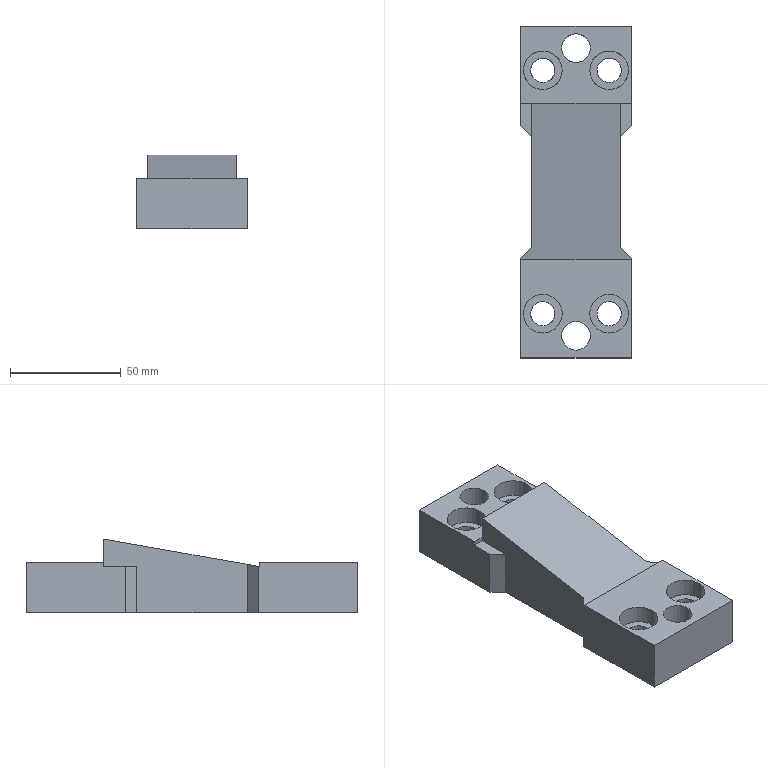Part | NX | features solid 2 | 1 solid | 36 faces | box 50 x 150 x 33.401 mm | volume 151864 mm3 | plane 26 | cylinder 10 | commonest cylinder face diameters 11 x4 17.5 x4 13 x2
STEP:
#1=CARTESIAN_POINT('',(-339.,-410.,-93.942));
#2=VERTEX_POINT('',#1);
#3=CARTESIAN_POINT('',(-339.,-410.329,-94.));
#4=VERTEX_POINT('',#3);
#5=CARTESIAN_POINT('',(-339.,-410.01,-93.944));
#6=DIRECTION('',(0.,-0.9848,-0.1736));
#7=VECTOR('',#6,1000.);
#8=LINE('',#5,#7);
#9=EDGE_CURVE('',#2,#4,#8,.T.);
#10=ORIENTED_EDGE('',*,*,#9,.F.);
#11=CARTESIAN_POINT('',(-339.,-410.,-115.));
#12=VERTEX_POINT('',#11);
#13=CARTESIAN_POINT('',(-339.,-410.,-94.));
#14=DIRECTION('',(0.,0.,-1.));
#15=VECTOR('',#14,1000.);
#16=LINE('',#13,#15);
#17=EDGE_CURVE('',#2,#12,#16,.T.);
#18=ORIENTED_EDGE('',*,*,#17,.T.);
#19=CARTESIAN_POINT('',(-339.,-455.,-115.));
#20=VERTEX_POINT('',#19);
#21=CARTESIAN_POINT('',(-339.,-410.,-115.));
#22=DIRECTION('',(0.,-1.,0.));
#23=VECTOR('',#22,1000.);
#24=LINE('',#21,#23);
#25=EDGE_CURVE('',#12,#20,#24,.T.);
#26=ORIENTED_EDGE('',*,*,#25,.T.);
#27=CARTESIAN_POINT('',(-339.,-455.,-92.));
#28=VERTEX_POINT('',#27);
#29=CARTESIAN_POINT('',(-339.,-455.,-94.));
#30=DIRECTION('',(0.,0.,-1.));
#31=VECTOR('',#30,1000.);
#32=LINE('',#29,#31);
#33=EDGE_CURVE('',#28,#20,#32,.T.);
#34=ORIENTED_EDGE('',*,*,#33,.F.);
#35=CARTESIAN_POINT('',(-339.,-410.329,-92.));
#36=VERTEX_POINT('',#35);
#37=CARTESIAN_POINT('',(-339.,-410.,-92.));
#38=DIRECTION('',(0.,-1.,0.));
#39=VECTOR('',#38,1000.);
#40=LINE('',#37,#39);
#41=EDGE_CURVE('',#36,#28,#40,.T.);
#42=ORIENTED_EDGE('',*,*,#41,.F.);
#43=CARTESIAN_POINT('',(-339.,-410.329,-94.));
#44=DIRECTION('',(0.,0.,-1.));
#45=VECTOR('',#44,1000.);
#46=LINE('',#43,#45);
#47=EDGE_CURVE('',#36,#4,#46,.T.);
#48=ORIENTED_EDGE('',*,*,#47,.T.);
#49=EDGE_LOOP('',(#10,#18,#26,#34,#42,#48));
#50=FACE_BOUND('',#49,.T.);
#51=CARTESIAN_POINT('',(-339.,-410.,-94.));
#52=DIRECTION('',(1.,0.,0.));
#53=DIRECTION('',(0.,1.,0.));
#54=AXIS2_PLACEMENT_3D('',#51,#52,#53);
#55=PLANE('',#54);
#56=ADVANCED_FACE('',(#50),#55,.F.);
#57=CARTESIAN_POINT('',(-334.,-405.,-93.06));
#58=VERTEX_POINT('',#57);
#59=CARTESIAN_POINT('',(-334.082,-405.082,-93.075));
#60=DIRECTION('',(-0.7017,-0.7017,-0.1237));
#61=VECTOR('',#60,1000.);
#62=LINE('',#59,#61);
#63=EDGE_CURVE('',#58,#2,#62,.T.);
#64=ORIENTED_EDGE('',*,*,#63,.F.);
#65=CARTESIAN_POINT('',(-334.,-405.,-115.));
#66=VERTEX_POINT('',#65);
#67=CARTESIAN_POINT('',(-334.,-405.,-94.));
#68=DIRECTION('',(0.,0.,-1.));
#69=VECTOR('',#68,1000.);
#70=LINE('',#67,#69);
#71=EDGE_CURVE('',#58,#66,#70,.T.);
#72=ORIENTED_EDGE('',*,*,#71,.T.);
#73=CARTESIAN_POINT('',(-334.,-405.,-115.));
#74=DIRECTION('',(-0.7071,-0.7071,0.));
#75=VECTOR('',#74,1000.);
#76=LINE('',#73,#75);
#77=EDGE_CURVE('',#66,#12,#76,.T.);
#78=ORIENTED_EDGE('',*,*,#77,.T.);
#79=ORIENTED_EDGE('',*,*,#17,.F.);
#80=EDGE_LOOP('',(#64,#72,#78,#79));
#81=FACE_BOUND('',#80,.T.);
#82=CARTESIAN_POINT('',(-334.,-405.,-94.));
#83=DIRECTION('',(0.7071,-0.7071,0.));
#84=DIRECTION('',(0.7071,0.7071,0.));
#85=AXIS2_PLACEMENT_3D('',#82,#83,#84);
#86=PLANE('',#85);
#87=ADVANCED_FACE('',(#81),#86,.F.);
#88=CARTESIAN_POINT('',(-329.,-443.75,-92.));
#89=VERTEX_POINT('',#88);
#90=CARTESIAN_POINT('',(-329.,-435.,-92.));
#91=DIRECTION('',(0.,0.,1.));
#92=DIRECTION('',(0.,-1.,0.));
#93=AXIS2_PLACEMENT_3D('',#90,#91,#92);
#94=CIRCLE('',#93,8.75);
#95=EDGE_CURVE('',#89,#89,#94,.T.);
#96=ORIENTED_EDGE('',*,*,#95,.F.);
#97=EDGE_LOOP('',(#96));
#98=FACE_BOUND('',#97,.T.);
#99=CARTESIAN_POINT('',(-314.,-451.5,-92.));
#100=VERTEX_POINT('',#99);
#101=CARTESIAN_POINT('',(-314.,-445.,-92.));
#102=DIRECTION('',(0.,0.,1.));
#103=DIRECTION('',(0.,-1.,0.));
#104=AXIS2_PLACEMENT_3D('',#101,#102,#103);
#105=CIRCLE('',#104,6.5);
#106=EDGE_CURVE('',#100,#100,#105,.T.);
#107=ORIENTED_EDGE('',*,*,#106,.F.);
#108=EDGE_LOOP('',(#107));
#109=FACE_BOUND('',#108,.T.);
#110=CARTESIAN_POINT('',(-299.,-443.75,-92.));
#111=VERTEX_POINT('',#110);
#112=CARTESIAN_POINT('',(-299.,-435.,-92.));
#113=DIRECTION('',(0.,0.,1.));
#114=DIRECTION('',(0.,-1.,0.));
#115=AXIS2_PLACEMENT_3D('',#112,#113,#114);
#116=CIRCLE('',#115,8.75);
#117=EDGE_CURVE('',#111,#111,#116,.T.);
#118=ORIENTED_EDGE('',*,*,#117,.F.);
#119=EDGE_LOOP('',(#118));
#120=FACE_BOUND('',#119,.T.);
#121=CARTESIAN_POINT('',(-289.,-410.329,-92.));
#122=VERTEX_POINT('',#121);
#123=CARTESIAN_POINT('',(-294.,-410.329,-92.));
#124=DIRECTION('',(-1.,0.,0.));
#125=VECTOR('',#124,1000.);
#126=LINE('',#123,#125);
#127=EDGE_CURVE('',#122,#36,#126,.T.);
#128=ORIENTED_EDGE('',*,*,#127,.T.);
#129=ORIENTED_EDGE('',*,*,#41,.T.);
#130=CARTESIAN_POINT('',(-289.,-455.,-92.));
#131=VERTEX_POINT('',#130);
#132=CARTESIAN_POINT('',(-289.,-455.,-92.));
#133=DIRECTION('',(-1.,0.,0.));
#134=VECTOR('',#133,1000.);
#135=LINE('',#132,#134);
#136=EDGE_CURVE('',#131,#28,#135,.T.);
#137=ORIENTED_EDGE('',*,*,#136,.F.);
#138=CARTESIAN_POINT('',(-289.,-410.,-92.));
#139=DIRECTION('',(0.,-1.,0.));
#140=VECTOR('',#139,1000.);
#141=LINE('',#138,#140);
#142=EDGE_CURVE('',#122,#131,#141,.T.);
#143=ORIENTED_EDGE('',*,*,#142,.F.);
#144=EDGE_LOOP('',(#128,#129,#137,#143));
#145=FACE_BOUND('',#144,.T.);
#146=CARTESIAN_POINT('',(-289.,-305.,-92.));
#147=DIRECTION('',(0.,0.,-1.));
#148=DIRECTION('',(1.,0.,0.));
#149=AXIS2_PLACEMENT_3D('',#146,#147,#148);
#150=PLANE('',#149);
#151=ADVANCED_FACE('',(#98,#109,#120,#145),#150,.F.);
#152=ORIENTED_EDGE('',*,*,#71,.F.);
#153=CARTESIAN_POINT('',(-334.,-340.,-81.599));
#154=VERTEX_POINT('',#153);
#155=CARTESIAN_POINT('',(-334.,-340.,-81.599));
#156=DIRECTION('',(0.,-0.9848,-0.1736));
#157=VECTOR('',#156,1000.);
#158=LINE('',#155,#157);
#159=EDGE_CURVE('',#154,#58,#158,.T.);
#160=ORIENTED_EDGE('',*,*,#159,.F.);
#161=CARTESIAN_POINT('',(-334.,-340.,-92.));
#162=VERTEX_POINT('',#161);
#163=CARTESIAN_POINT('',(-334.,-340.,-81.599));
#164=DIRECTION('',(0.,0.,-1.));
#165=VECTOR('',#164,1000.);
#166=LINE('',#163,#165);
#167=EDGE_CURVE('',#154,#162,#166,.T.);
#168=ORIENTED_EDGE('',*,*,#167,.T.);
#169=CARTESIAN_POINT('',(-334.,-340.,-94.));
#170=VERTEX_POINT('',#169);
#171=CARTESIAN_POINT('',(-334.,-340.,-81.599));
#172=DIRECTION('',(0.,0.,-1.));
#173=VECTOR('',#172,1000.);
#174=LINE('',#171,#173);
#175=EDGE_CURVE('',#162,#170,#174,.T.);
#176=ORIENTED_EDGE('',*,*,#175,.T.);
#177=CARTESIAN_POINT('',(-334.,-355.,-94.));
#178=VERTEX_POINT('',#177);
#179=CARTESIAN_POINT('',(-334.,-340.,-94.));
#180=DIRECTION('',(0.,-1.,0.));
#181=VECTOR('',#180,1000.);
#182=LINE('',#179,#181);
#183=EDGE_CURVE('',#170,#178,#182,.T.);
#184=ORIENTED_EDGE('',*,*,#183,.T.);
#185=CARTESIAN_POINT('',(-334.,-355.,-115.));
#186=VERTEX_POINT('',#185);
#187=CARTESIAN_POINT('',(-334.,-355.,-94.));
#188=DIRECTION('',(0.,0.,-1.));
#189=VECTOR('',#188,1000.);
#190=LINE('',#187,#189);
#191=EDGE_CURVE('',#178,#186,#190,.T.);
#192=ORIENTED_EDGE('',*,*,#191,.T.);
#193=CARTESIAN_POINT('',(-334.,-355.,-115.));
#194=DIRECTION('',(0.,-1.,0.));
#195=VECTOR('',#194,1000.);
#196=LINE('',#193,#195);
#197=EDGE_CURVE('',#186,#66,#196,.T.);
#198=ORIENTED_EDGE('',*,*,#197,.T.);
#199=EDGE_LOOP('',(#152,#160,#168,#176,#184,#192,#198));
#200=FACE_BOUND('',#199,.T.);
#201=CARTESIAN_POINT('',(-334.,-355.,-94.));
#202=DIRECTION('',(1.,0.,0.));
#203=DIRECTION('',(0.,1.,0.));
#204=AXIS2_PLACEMENT_3D('',#201,#202,#203);
#205=PLANE('',#204);
#206=ADVANCED_FACE('',(#200),#205,.F.);
#207=CARTESIAN_POINT('',(-294.,-340.,-81.599));
#208=VERTEX_POINT('',#207);
#209=CARTESIAN_POINT('',(-294.,-340.,-92.));
#210=VERTEX_POINT('',#209);
#211=CARTESIAN_POINT('',(-294.,-340.,-81.599));
#212=DIRECTION('',(0.,0.,-1.));
#213=VECTOR('',#212,1000.);
#214=LINE('',#211,#213);
#215=EDGE_CURVE('',#208,#210,#214,.T.);
#216=ORIENTED_EDGE('',*,*,#215,.T.);
#217=CARTESIAN_POINT('',(-294.,-340.,-92.));
#218=DIRECTION('',(-1.,0.,0.));
#219=VECTOR('',#218,1000.);
#220=LINE('',#217,#219);
#221=EDGE_CURVE('',#210,#162,#220,.T.);
#222=ORIENTED_EDGE('',*,*,#221,.T.);
#223=ORIENTED_EDGE('',*,*,#167,.F.);
#224=CARTESIAN_POINT('',(-294.,-340.,-81.599));
#225=DIRECTION('',(-1.,0.,0.));
#226=VECTOR('',#225,1000.);
#227=LINE('',#224,#226);
#228=EDGE_CURVE('',#208,#154,#227,.T.);
#229=ORIENTED_EDGE('',*,*,#228,.F.);
#230=EDGE_LOOP('',(#216,#222,#223,#229));
#231=FACE_BOUND('',#230,.T.);
#232=CARTESIAN_POINT('',(-294.,-340.,-81.599));
#233=DIRECTION('',(0.,1.,0.));
#234=DIRECTION('',(-1.,0.,0.));
#235=AXIS2_PLACEMENT_3D('',#232,#233,#234);
#236=PLANE('',#235);
#237=ADVANCED_FACE('',(#231),#236,.T.);
#238=ORIENTED_EDGE('',*,*,#183,.F.);
#239=CARTESIAN_POINT('',(-339.,-340.,-94.));
#240=VERTEX_POINT('',#239);
#241=CARTESIAN_POINT('',(-289.,-340.,-94.));
#242=DIRECTION('',(-1.,0.,0.));
#243=VECTOR('',#242,1000.);
#244=LINE('',#241,#243);
#245=EDGE_CURVE('',#170,#240,#244,.T.);
#246=ORIENTED_EDGE('',*,*,#245,.T.);
#247=CARTESIAN_POINT('',(-339.,-350.,-94.));
#248=VERTEX_POINT('',#247);
#249=CARTESIAN_POINT('',(-339.,-305.,-94.));
#250=DIRECTION('',(0.,-1.,0.));
#251=VECTOR('',#250,1000.);
#252=LINE('',#249,#251);
#253=EDGE_CURVE('',#240,#248,#252,.T.);
#254=ORIENTED_EDGE('',*,*,#253,.T.);
#255=CARTESIAN_POINT('',(-334.,-355.,-94.));
#256=DIRECTION('',(-0.7071,0.7071,0.));
#257=VECTOR('',#256,1000.);
#258=LINE('',#255,#257);
#259=EDGE_CURVE('',#178,#248,#258,.T.);
#260=ORIENTED_EDGE('',*,*,#259,.F.);
#261=EDGE_LOOP('',(#238,#246,#254,#260));
#262=FACE_BOUND('',#261,.T.);
#263=CARTESIAN_POINT('',(-289.,-305.,-94.));
#264=DIRECTION('',(0.,0.,-1.));
#265=DIRECTION('',(1.,0.,0.));
#266=AXIS2_PLACEMENT_3D('',#263,#264,#265);
#267=PLANE('',#266);
#268=ADVANCED_FACE('',(#262),#267,.F.);
#269=CARTESIAN_POINT('',(-289.,-340.,-94.));
#270=VERTEX_POINT('',#269);
#271=CARTESIAN_POINT('',(-294.,-340.,-94.));
#272=VERTEX_POINT('',#271);
#273=CARTESIAN_POINT('',(-289.,-340.,-94.));
#274=DIRECTION('',(-1.,0.,0.));
#275=VECTOR('',#274,1000.);
#276=LINE('',#273,#275);
#277=EDGE_CURVE('',#270,#272,#276,.T.);
#278=ORIENTED_EDGE('',*,*,#277,.T.);
#279=CARTESIAN_POINT('',(-294.,-355.,-94.));
#280=VERTEX_POINT('',#279);
#281=CARTESIAN_POINT('',(-294.,-340.,-94.));
#282=DIRECTION('',(0.,-1.,0.));
#283=VECTOR('',#282,1000.);
#284=LINE('',#281,#283);
#285=EDGE_CURVE('',#272,#280,#284,.T.);
#286=ORIENTED_EDGE('',*,*,#285,.T.);
#287=CARTESIAN_POINT('',(-289.,-350.,-94.));
#288=VERTEX_POINT('',#287);
#289=CARTESIAN_POINT('',(-289.,-350.,-94.));
#290=DIRECTION('',(-0.7071,-0.7071,0.));
#291=VECTOR('',#290,1000.);
#292=LINE('',#289,#291);
#293=EDGE_CURVE('',#288,#280,#292,.T.);
#294=ORIENTED_EDGE('',*,*,#293,.F.);
#295=CARTESIAN_POINT('',(-289.,-305.,-94.));
#296=DIRECTION('',(0.,-1.,0.));
#297=VECTOR('',#296,1000.);
#298=LINE('',#295,#297);
#299=EDGE_CURVE('',#270,#288,#298,.T.);
#300=ORIENTED_EDGE('',*,*,#299,.F.);
#301=EDGE_LOOP('',(#278,#286,#294,#300));
#302=FACE_BOUND('',#301,.T.);
#303=CARTESIAN_POINT('',(-289.,-305.,-94.));
#304=DIRECTION('',(0.,0.,-1.));
#305=DIRECTION('',(1.,0.,0.));
#306=AXIS2_PLACEMENT_3D('',#303,#304,#305);
#307=PLANE('',#306);
#308=ADVANCED_FACE('',(#302),#307,.F.);
#309=ORIENTED_EDGE('',*,*,#245,.F.);
#310=ORIENTED_EDGE('',*,*,#175,.F.);
#311=CARTESIAN_POINT('',(-339.,-340.,-92.));
#312=VERTEX_POINT('',#311);
#313=CARTESIAN_POINT('',(-289.,-340.,-92.));
#314=DIRECTION('',(-1.,0.,0.));
#315=VECTOR('',#314,1000.);
#316=LINE('',#313,#315);
#317=EDGE_CURVE('',#162,#312,#316,.T.);
#318=ORIENTED_EDGE('',*,*,#317,.T.);
#319=CARTESIAN_POINT('',(-339.,-340.,-94.));
#320=DIRECTION('',(0.,0.,-1.));
#321=VECTOR('',#320,1000.);
#322=LINE('',#319,#321);
#323=EDGE_CURVE('',#312,#240,#322,.T.);
#324=ORIENTED_EDGE('',*,*,#323,.T.);
#325=EDGE_LOOP('',(#309,#310,#318,#324));
#326=FACE_BOUND('',#325,.T.);
#327=CARTESIAN_POINT('',(-289.,-340.,-75.44));
#328=DIRECTION('',(0.,-1.,0.));
#329=DIRECTION('',(1.,0.,0.));
#330=AXIS2_PLACEMENT_3D('',#327,#328,#329);
#331=PLANE('',#330);
#332=ADVANCED_FACE('',(#326),#331,.T.);
#333=CARTESIAN_POINT('',(-329.,-440.5,-115.));
#334=VERTEX_POINT('',#333);
#335=CARTESIAN_POINT('',(-329.,-435.,-115.));
#336=DIRECTION('',(0.,0.,1.));
#337=DIRECTION('',(0.,-1.,0.));
#338=AXIS2_PLACEMENT_3D('',#335,#336,#337);
#339=CIRCLE('',#338,5.5);
#340=EDGE_CURVE('',#334,#334,#339,.T.);
#341=ORIENTED_EDGE('',*,*,#340,.F.);
#342=EDGE_LOOP('',(#341));
#343=FACE_BOUND('',#342,.T.);
#344=CARTESIAN_POINT('',(-334.5,-435.,-100.));
#345=VERTEX_POINT('',#344);
#346=CARTESIAN_POINT('',(-329.,-435.,-100.));
#347=DIRECTION('',(0.,0.,1.));
#348=DIRECTION('',(-1.,0.,0.));
#349=AXIS2_PLACEMENT_3D('',#346,#347,#348);
#350=CIRCLE('',#349,5.5);
#351=EDGE_CURVE('',#345,#345,#350,.T.);
#352=ORIENTED_EDGE('',*,*,#351,.T.);
#353=EDGE_LOOP('',(#352));
#354=FACE_BOUND('',#353,.T.);
#355=CARTESIAN_POINT('',(-329.,-435.,-94.));
#356=DIRECTION('',(0.,0.,-1.));
#357=DIRECTION('',(1.,0.,0.));
#358=AXIS2_PLACEMENT_3D('',#355,#356,#357);
#359=CYLINDRICAL_SURFACE('',#358,5.5);
#360=ADVANCED_FACE('',(#343,#354),#359,.F.);
#361=CARTESIAN_POINT('',(-299.,-440.5,-115.));
#362=VERTEX_POINT('',#361);
#363=CARTESIAN_POINT('',(-299.,-435.,-115.));
#364=DIRECTION('',(0.,0.,1.));
#365=DIRECTION('',(0.,-1.,0.));
#366=AXIS2_PLACEMENT_3D('',#363,#364,#365);
#367=CIRCLE('',#366,5.5);
#368=EDGE_CURVE('',#362,#362,#367,.T.);
#369=ORIENTED_EDGE('',*,*,#368,.F.);
#370=EDGE_LOOP('',(#369));
#371=FACE_BOUND('',#370,.T.);
#372=CARTESIAN_POINT('',(-304.5,-435.,-100.));
#373=VERTEX_POINT('',#372);
#374=CARTESIAN_POINT('',(-299.,-435.,-100.));
#375=DIRECTION('',(0.,0.,1.));
#376=DIRECTION('',(-1.,0.,0.));
#377=AXIS2_PLACEMENT_3D('',#374,#375,#376);
#378=CIRCLE('',#377,5.5);
#379=EDGE_CURVE('',#373,#373,#378,.T.);
#380=ORIENTED_EDGE('',*,*,#379,.T.);
#381=EDGE_LOOP('',(#380));
#382=FACE_BOUND('',#381,.T.);
#383=CARTESIAN_POINT('',(-299.,-435.,-94.));
#384=DIRECTION('',(0.,0.,-1.));
#385=DIRECTION('',(1.,0.,0.));
#386=AXIS2_PLACEMENT_3D('',#383,#384,#385);
#387=CYLINDRICAL_SURFACE('',#386,5.5);
#388=ADVANCED_FACE('',(#371,#382),#387,.F.);
#389=CARTESIAN_POINT('',(-339.,-305.,-115.));
#390=VERTEX_POINT('',#389);
#391=CARTESIAN_POINT('',(-339.,-350.,-115.));
#392=VERTEX_POINT('',#391);
#393=CARTESIAN_POINT('',(-339.,-305.,-115.));
#394=DIRECTION('',(0.,-1.,0.));
#395=VECTOR('',#394,1000.);
#396=LINE('',#393,#395);
#397=EDGE_CURVE('',#390,#392,#396,.T.);
#398=ORIENTED_EDGE('',*,*,#397,.F.);
#399=CARTESIAN_POINT('',(-289.,-305.,-115.));
#400=VERTEX_POINT('',#399);
#401=CARTESIAN_POINT('',(-339.,-305.,-115.));
#402=DIRECTION('',(1.,0.,0.));
#403=VECTOR('',#402,1000.);
#404=LINE('',#401,#403);
#405=EDGE_CURVE('',#390,#400,#404,.T.);
#406=ORIENTED_EDGE('',*,*,#405,.T.);
#407=CARTESIAN_POINT('',(-289.,-350.,-115.));
#408=VERTEX_POINT('',#407);
#409=CARTESIAN_POINT('',(-289.,-305.,-115.));
#410=DIRECTION('',(0.,-1.,0.));
#411=VECTOR('',#410,1000.);
#412=LINE('',#409,#411);
#413=EDGE_CURVE('',#400,#408,#412,.T.);
#414=ORIENTED_EDGE('',*,*,#413,.T.);
#415=CARTESIAN_POINT('',(-294.,-355.,-115.));
#416=VERTEX_POINT('',#415);
#417=CARTESIAN_POINT('',(-289.,-350.,-115.));
#418=DIRECTION('',(-0.7071,-0.7071,0.));
#419=VECTOR('',#418,1000.);
#420=LINE('',#417,#419);
#421=EDGE_CURVE('',#408,#416,#420,.T.);
#422=ORIENTED_EDGE('',*,*,#421,.T.);
#423=CARTESIAN_POINT('',(-294.,-405.,-115.));
#424=VERTEX_POINT('',#423);
#425=CARTESIAN_POINT('',(-294.,-355.,-115.));
#426=DIRECTION('',(0.,-1.,0.));
#427=VECTOR('',#426,1000.);
#428=LINE('',#425,#427);
#429=EDGE_CURVE('',#416,#424,#428,.T.);
#430=ORIENTED_EDGE('',*,*,#429,.T.);
#431=CARTESIAN_POINT('',(-289.,-410.,-115.));
#432=VERTEX_POINT('',#431);
#433=CARTESIAN_POINT('',(-294.,-405.,-115.));
#434=DIRECTION('',(0.7071,-0.7071,0.));
#435=VECTOR('',#434,1000.);
#436=LINE('',#433,#435);
#437=EDGE_CURVE('',#424,#432,#436,.T.);
#438=ORIENTED_EDGE('',*,*,#437,.T.);
#439=CARTESIAN_POINT('',(-289.,-455.,-115.));
#440=VERTEX_POINT('',#439);
#441=CARTESIAN_POINT('',(-289.,-410.,-115.));
#442=DIRECTION('',(0.,-1.,0.));
#443=VECTOR('',#442,1000.);
#444=LINE('',#441,#443);
#445=EDGE_CURVE('',#432,#440,#444,.T.);
#446=ORIENTED_EDGE('',*,*,#445,.T.);
#447=CARTESIAN_POINT('',(-289.,-455.,-115.));
#448=DIRECTION('',(-1.,0.,0.));
#449=VECTOR('',#448,1000.);
#450=LINE('',#447,#449);
#451=EDGE_CURVE('',#440,#20,#450,.T.);
#452=ORIENTED_EDGE('',*,*,#451,.T.);
#453=ORIENTED_EDGE('',*,*,#25,.F.);
#454=ORIENTED_EDGE('',*,*,#77,.F.);
#455=ORIENTED_EDGE('',*,*,#197,.F.);
#456=CARTESIAN_POINT('',(-334.,-355.,-115.));
#457=DIRECTION('',(-0.7071,0.7071,0.));
#458=VECTOR('',#457,1000.);
#459=LINE('',#456,#458);
#460=EDGE_CURVE('',#186,#392,#459,.T.);
#461=ORIENTED_EDGE('',*,*,#460,.T.);
#462=EDGE_LOOP('',(#398,#406,#414,#422,#430,#438,#446,#452,#453,#454,#455,#461));
#463=FACE_BOUND('',#462,.T.);
#464=ORIENTED_EDGE('',*,*,#340,.T.);
#465=EDGE_LOOP('',(#464));
#466=FACE_BOUND('',#465,.T.);
#467=ORIENTED_EDGE('',*,*,#368,.T.);
#468=EDGE_LOOP('',(#467));
#469=FACE_BOUND('',#468,.T.);
#470=CARTESIAN_POINT('',(-314.,-451.5,-115.));
#471=VERTEX_POINT('',#470);
#472=CARTESIAN_POINT('',(-314.,-445.,-115.));
#473=DIRECTION('',(0.,0.,1.));
#474=DIRECTION('',(0.,-1.,0.));
#475=AXIS2_PLACEMENT_3D('',#472,#473,#474);
#476=CIRCLE('',#475,6.5);
#477=EDGE_CURVE('',#471,#471,#476,.T.);
#478=ORIENTED_EDGE('',*,*,#477,.T.);
#479=EDGE_LOOP('',(#478));
#480=FACE_BOUND('',#479,.T.);
#481=CARTESIAN_POINT('',(-329.,-330.5,-115.));
#482=VERTEX_POINT('',#481);
#483=CARTESIAN_POINT('',(-329.,-325.,-115.));
#484=DIRECTION('',(0.,0.,1.));
#485=DIRECTION('',(0.,-1.,0.));
#486=AXIS2_PLACEMENT_3D('',#483,#484,#485);
#487=CIRCLE('',#486,5.5);
#488=EDGE_CURVE('',#482,#482,#487,.T.);
#489=ORIENTED_EDGE('',*,*,#488,.T.);
#490=EDGE_LOOP('',(#489));
#491=FACE_BOUND('',#490,.T.);
#492=CARTESIAN_POINT('',(-299.,-330.5,-115.));
#493=VERTEX_POINT('',#492);
#494=CARTESIAN_POINT('',(-299.,-325.,-115.));
#495=DIRECTION('',(0.,0.,1.));
#496=DIRECTION('',(0.,-1.,0.));
#497=AXIS2_PLACEMENT_3D('',#494,#495,#496);
#498=CIRCLE('',#497,5.5);
#499=EDGE_CURVE('',#493,#493,#498,.T.);
#500=ORIENTED_EDGE('',*,*,#499,.T.);
#501=EDGE_LOOP('',(#500));
#502=FACE_BOUND('',#501,.T.);
#503=CARTESIAN_POINT('',(-314.,-321.5,-115.));
#504=VERTEX_POINT('',#503);
#505=CARTESIAN_POINT('',(-314.,-315.,-115.));
#506=DIRECTION('',(0.,0.,1.));
#507=DIRECTION('',(0.,-1.,0.));
#508=AXIS2_PLACEMENT_3D('',#505,#506,#507);
#509=CIRCLE('',#508,6.5);
#510=EDGE_CURVE('',#504,#504,#509,.T.);
#511=ORIENTED_EDGE('',*,*,#510,.T.);
#512=EDGE_LOOP('',(#511));
#513=FACE_BOUND('',#512,.T.);
#514=CARTESIAN_POINT('',(-289.,-305.,-115.));
#515=DIRECTION('',(0.,0.,-1.));
#516=DIRECTION('',(1.,0.,0.));
#517=AXIS2_PLACEMENT_3D('',#514,#515,#516);
#518=PLANE('',#517);
#519=ADVANCED_FACE('',(#463,#466,#469,#480,#491,#502,#513),#518,.T.);
#520=ORIENTED_EDGE('',*,*,#413,.F.);
#521=CARTESIAN_POINT('',(-289.,-305.,-92.));
#522=VERTEX_POINT('',#521);
#523=CARTESIAN_POINT('',(-289.,-305.,-94.));
#524=DIRECTION('',(0.,0.,-1.));
#525=VECTOR('',#524,1000.);
#526=LINE('',#523,#525);
#527=EDGE_CURVE('',#522,#400,#526,.T.);
#528=ORIENTED_EDGE('',*,*,#527,.F.);
#529=CARTESIAN_POINT('',(-289.,-340.,-92.));
#530=VERTEX_POINT('',#529);
#531=CARTESIAN_POINT('',(-289.,-305.,-92.));
#532=DIRECTION('',(0.,-1.,0.));
#533=VECTOR('',#532,1000.);
#534=LINE('',#531,#533);
#535=EDGE_CURVE('',#522,#530,#534,.T.);
#536=ORIENTED_EDGE('',*,*,#535,.T.);
#537=CARTESIAN_POINT('',(-289.,-340.,-94.));
#538=DIRECTION('',(0.,0.,-1.));
#539=VECTOR('',#538,1000.);
#540=LINE('',#537,#539);
#541=EDGE_CURVE('',#530,#270,#540,.T.);
#542=ORIENTED_EDGE('',*,*,#541,.T.);
#543=ORIENTED_EDGE('',*,*,#299,.T.);
#544=CARTESIAN_POINT('',(-289.,-350.,-94.));
#545=DIRECTION('',(0.,0.,-1.));
#546=VECTOR('',#545,1000.);
#547=LINE('',#544,#546);
#548=EDGE_CURVE('',#288,#408,#547,.T.);
#549=ORIENTED_EDGE('',*,*,#548,.T.);
#550=EDGE_LOOP('',(#520,#528,#536,#542,#543,#549));
#551=FACE_BOUND('',#550,.T.);
#552=CARTESIAN_POINT('',(-289.,-305.,-94.));
#553=DIRECTION('',(1.,0.,0.));
#554=DIRECTION('',(0.,1.,0.));
#555=AXIS2_PLACEMENT_3D('',#552,#553,#554);
#556=PLANE('',#555);
#557=ADVANCED_FACE('',(#551),#556,.T.);
#558=ORIENTED_EDGE('',*,*,#421,.F.);
#559=ORIENTED_EDGE('',*,*,#548,.F.);
#560=ORIENTED_EDGE('',*,*,#293,.T.);
#561=CARTESIAN_POINT('',(-294.,-355.,-94.));
#562=DIRECTION('',(0.,0.,-1.));
#563=VECTOR('',#562,1000.);
#564=LINE('',#561,#563);
#565=EDGE_CURVE('',#280,#416,#564,.T.);
#566=ORIENTED_EDGE('',*,*,#565,.T.);
#567=EDGE_LOOP('',(#558,#559,#560,#566));
#568=FACE_BOUND('',#567,.T.);
#569=CARTESIAN_POINT('',(-289.,-350.,-94.));
#570=DIRECTION('',(0.7071,-0.7071,0.));
#571=DIRECTION('',(0.7071,0.7071,0.));
#572=AXIS2_PLACEMENT_3D('',#569,#570,#571);
#573=PLANE('',#572);
#574=ADVANCED_FACE('',(#568),#573,.T.);
#575=CARTESIAN_POINT('',(-294.,-405.,-93.06));
#576=VERTEX_POINT('',#575);
#577=CARTESIAN_POINT('',(-294.,-340.,-81.599));
#578=DIRECTION('',(0.,-0.9848,-0.1736));
#579=VECTOR('',#578,1000.);
#580=LINE('',#577,#579);
#581=EDGE_CURVE('',#208,#576,#580,.T.);
#582=ORIENTED_EDGE('',*,*,#581,.T.);
#583=CARTESIAN_POINT('',(-294.,-405.,-94.));
#584=DIRECTION('',(0.,0.,-1.));
#585=VECTOR('',#584,1000.);
#586=LINE('',#583,#585);
#587=EDGE_CURVE('',#576,#424,#586,.T.);
#588=ORIENTED_EDGE('',*,*,#587,.T.);
#589=ORIENTED_EDGE('',*,*,#429,.F.);
#590=ORIENTED_EDGE('',*,*,#565,.F.);
#591=ORIENTED_EDGE('',*,*,#285,.F.);
#592=CARTESIAN_POINT('',(-294.,-340.,-81.599));
#593=DIRECTION('',(0.,0.,-1.));
#594=VECTOR('',#593,1000.);
#595=LINE('',#592,#594);
#596=EDGE_CURVE('',#210,#272,#595,.T.);
#597=ORIENTED_EDGE('',*,*,#596,.F.);
#598=ORIENTED_EDGE('',*,*,#215,.F.);
#599=EDGE_LOOP('',(#582,#588,#589,#590,#591,#597,#598));
#600=FACE_BOUND('',#599,.T.);
#601=CARTESIAN_POINT('',(-294.,-355.,-94.));
#602=DIRECTION('',(1.,0.,0.));
#603=DIRECTION('',(0.,1.,0.));
#604=AXIS2_PLACEMENT_3D('',#601,#602,#603);
#605=PLANE('',#604);
#606=ADVANCED_FACE('',(#600),#605,.T.);
#607=CARTESIAN_POINT('',(-289.,-410.,-93.942));
#608=VERTEX_POINT('',#607);
#609=CARTESIAN_POINT('',(-293.918,-405.082,-93.075));
#610=DIRECTION('',(-0.7017,0.7017,0.1237));
#611=VECTOR('',#610,1000.);
#612=LINE('',#609,#611);
#613=EDGE_CURVE('',#608,#576,#612,.T.);
#614=ORIENTED_EDGE('',*,*,#613,.F.);
#615=CARTESIAN_POINT('',(-289.,-410.,-94.));
#616=DIRECTION('',(0.,0.,-1.));
#617=VECTOR('',#616,1000.);
#618=LINE('',#615,#617);
#619=EDGE_CURVE('',#608,#432,#618,.T.);
#620=ORIENTED_EDGE('',*,*,#619,.T.);
#621=ORIENTED_EDGE('',*,*,#437,.F.);
#622=ORIENTED_EDGE('',*,*,#587,.F.);
#623=EDGE_LOOP('',(#614,#620,#621,#622));
#624=FACE_BOUND('',#623,.T.);
#625=CARTESIAN_POINT('',(-294.,-405.,-94.));
#626=DIRECTION('',(0.7071,0.7071,0.));
#627=DIRECTION('',(-0.7071,0.7071,0.));
#628=AXIS2_PLACEMENT_3D('',#625,#626,#627);
#629=PLANE('',#628);
#630=ADVANCED_FACE('',(#624),#629,.T.);
#631=CARTESIAN_POINT('',(-289.,-410.329,-94.));
#632=VERTEX_POINT('',#631);
#633=CARTESIAN_POINT('',(-289.,-410.01,-93.944));
#634=DIRECTION('',(0.,0.9848,0.1736));
#635=VECTOR('',#634,1000.);
#636=LINE('',#633,#635);
#637=EDGE_CURVE('',#632,#608,#636,.T.);
#638=ORIENTED_EDGE('',*,*,#637,.F.);
#639=CARTESIAN_POINT('',(-289.,-410.329,-94.));
#640=DIRECTION('',(0.,0.,1.));
#641=VECTOR('',#640,1000.);
#642=LINE('',#639,#641);
#643=EDGE_CURVE('',#632,#122,#642,.T.);
#644=ORIENTED_EDGE('',*,*,#643,.T.);
#645=ORIENTED_EDGE('',*,*,#142,.T.);
#646=CARTESIAN_POINT('',(-289.,-455.,-94.));
#647=DIRECTION('',(0.,0.,-1.));
#648=VECTOR('',#647,1000.);
#649=LINE('',#646,#648);
#650=EDGE_CURVE('',#131,#440,#649,.T.);
#651=ORIENTED_EDGE('',*,*,#650,.T.);
#652=ORIENTED_EDGE('',*,*,#445,.F.);
#653=ORIENTED_EDGE('',*,*,#619,.F.);
#654=EDGE_LOOP('',(#638,#644,#645,#651,#652,#653));
#655=FACE_BOUND('',#654,.T.);
#656=CARTESIAN_POINT('',(-289.,-410.,-94.));
#657=DIRECTION('',(1.,0.,0.));
#658=DIRECTION('',(0.,1.,0.));
#659=AXIS2_PLACEMENT_3D('',#656,#657,#658);
#660=PLANE('',#659);
#661=ADVANCED_FACE('',(#655),#660,.T.);
#662=ORIENTED_EDGE('',*,*,#451,.F.);
#663=ORIENTED_EDGE('',*,*,#650,.F.);
#664=ORIENTED_EDGE('',*,*,#136,.T.);
#665=ORIENTED_EDGE('',*,*,#33,.T.);
#666=EDGE_LOOP('',(#662,#663,#664,#665));
#667=FACE_BOUND('',#666,.T.);
#668=CARTESIAN_POINT('',(-289.,-455.,-94.));
#669=DIRECTION('',(0.,-1.,0.));
#670=DIRECTION('',(1.,0.,0.));
#671=AXIS2_PLACEMENT_3D('',#668,#669,#670);
#672=PLANE('',#671);
#673=ADVANCED_FACE('',(#667),#672,.T.);
#674=ORIENTED_EDGE('',*,*,#460,.F.);
#675=ORIENTED_EDGE('',*,*,#191,.F.);
#676=ORIENTED_EDGE('',*,*,#259,.T.);
#677=CARTESIAN_POINT('',(-339.,-350.,-94.));
#678=DIRECTION('',(0.,0.,-1.));
#679=VECTOR('',#678,1000.);
#680=LINE('',#677,#679);
#681=EDGE_CURVE('',#248,#392,#680,.T.);
#682=ORIENTED_EDGE('',*,*,#681,.T.);
#683=EDGE_LOOP('',(#674,#675,#676,#682));
#684=FACE_BOUND('',#683,.T.);
#685=CARTESIAN_POINT('',(-334.,-355.,-94.));
#686=DIRECTION('',(-0.7071,-0.7071,0.));
#687=DIRECTION('',(0.7071,-0.7071,0.));
#688=AXIS2_PLACEMENT_3D('',#685,#686,#687);
#689=PLANE('',#688);
#690=ADVANCED_FACE('',(#684),#689,.T.);
#691=ORIENTED_EDGE('',*,*,#253,.F.);
#692=ORIENTED_EDGE('',*,*,#323,.F.);
#693=CARTESIAN_POINT('',(-339.,-305.,-92.));
#694=VERTEX_POINT('',#693);
#695=CARTESIAN_POINT('',(-339.,-305.,-92.));
#696=DIRECTION('',(0.,-1.,0.));
#697=VECTOR('',#696,1000.);
#698=LINE('',#695,#697);
#699=EDGE_CURVE('',#694,#312,#698,.T.);
#700=ORIENTED_EDGE('',*,*,#699,.F.);
#701=CARTESIAN_POINT('',(-339.,-305.,-94.));
#702=DIRECTION('',(0.,0.,-1.));
#703=VECTOR('',#702,1000.);
#704=LINE('',#701,#703);
#705=EDGE_CURVE('',#694,#390,#704,.T.);
#706=ORIENTED_EDGE('',*,*,#705,.T.);
#707=ORIENTED_EDGE('',*,*,#397,.T.);
#708=ORIENTED_EDGE('',*,*,#681,.F.);
#709=EDGE_LOOP('',(#691,#692,#700,#706,#707,#708));
#710=FACE_BOUND('',#709,.T.);
#711=CARTESIAN_POINT('',(-339.,-305.,-94.));
#712=DIRECTION('',(1.,0.,0.));
#713=DIRECTION('',(0.,1.,0.));
#714=AXIS2_PLACEMENT_3D('',#711,#712,#713);
#715=PLANE('',#714);
#716=ADVANCED_FACE('',(#710),#715,.F.);
#717=ORIENTED_EDGE('',*,*,#477,.F.);
#718=EDGE_LOOP('',(#717));
#719=FACE_BOUND('',#718,.T.);
#720=ORIENTED_EDGE('',*,*,#106,.T.);
#721=EDGE_LOOP('',(#720));
#722=FACE_BOUND('',#721,.T.);
#723=CARTESIAN_POINT('',(-314.,-445.,-94.));
#724=DIRECTION('',(0.,0.,-1.));
#725=DIRECTION('',(1.,0.,0.));
#726=AXIS2_PLACEMENT_3D('',#723,#724,#725);
#727=CYLINDRICAL_SURFACE('',#726,6.5);
#728=ADVANCED_FACE('',(#719,#722),#727,.F.);
#729=CARTESIAN_POINT('',(-299.,-443.75,-100.));
#730=VERTEX_POINT('',#729);
#731=CARTESIAN_POINT('',(-299.,-435.,-100.));
#732=DIRECTION('',(0.,0.,1.));
#733=DIRECTION('',(0.,-1.,0.));
#734=AXIS2_PLACEMENT_3D('',#731,#732,#733);
#735=CIRCLE('',#734,8.75);
#736=EDGE_CURVE('',#730,#730,#735,.T.);
#737=ORIENTED_EDGE('',*,*,#736,.F.);
#738=EDGE_LOOP('',(#737));
#739=FACE_BOUND('',#738,.T.);
#740=ORIENTED_EDGE('',*,*,#117,.T.);
#741=EDGE_LOOP('',(#740));
#742=FACE_BOUND('',#741,.T.);
#743=CARTESIAN_POINT('',(-299.,-435.,-94.));
#744=DIRECTION('',(0.,0.,-1.));
#745=DIRECTION('',(1.,0.,0.));
#746=AXIS2_PLACEMENT_3D('',#743,#744,#745);
#747=CYLINDRICAL_SURFACE('',#746,8.75);
#748=ADVANCED_FACE('',(#739,#742),#747,.F.);
#749=ORIENTED_EDGE('',*,*,#379,.F.);
#750=EDGE_LOOP('',(#749));
#751=FACE_BOUND('',#750,.T.);
#752=ORIENTED_EDGE('',*,*,#736,.T.);
#753=EDGE_LOOP('',(#752));
#754=FACE_BOUND('',#753,.T.);
#755=CARTESIAN_POINT('',(-299.,-435.,-100.));
#756=DIRECTION('',(0.,0.,1.));
#757=DIRECTION('',(-1.,0.,0.));
#758=AXIS2_PLACEMENT_3D('',#755,#756,#757);
#759=PLANE('',#758);
#760=ADVANCED_FACE('',(#751,#754),#759,.T.);
#761=CARTESIAN_POINT('',(-329.,-443.75,-100.));
#762=VERTEX_POINT('',#761);
#763=CARTESIAN_POINT('',(-329.,-435.,-100.));
#764=DIRECTION('',(0.,0.,1.));
#765=DIRECTION('',(0.,-1.,0.));
#766=AXIS2_PLACEMENT_3D('',#763,#764,#765);
#767=CIRCLE('',#766,8.75);
#768=EDGE_CURVE('',#762,#762,#767,.T.);
#769=ORIENTED_EDGE('',*,*,#768,.F.);
#770=EDGE_LOOP('',(#769));
#771=FACE_BOUND('',#770,.T.);
#772=ORIENTED_EDGE('',*,*,#95,.T.);
#773=EDGE_LOOP('',(#772));
#774=FACE_BOUND('',#773,.T.);
#775=CARTESIAN_POINT('',(-329.,-435.,-94.));
#776=DIRECTION('',(0.,0.,-1.));
#777=DIRECTION('',(1.,0.,0.));
#778=AXIS2_PLACEMENT_3D('',#775,#776,#777);
#779=CYLINDRICAL_SURFACE('',#778,8.75);
#780=ADVANCED_FACE('',(#771,#774),#779,.F.);
#781=ORIENTED_EDGE('',*,*,#351,.F.);
#782=EDGE_LOOP('',(#781));
#783=FACE_BOUND('',#782,.T.);
#784=ORIENTED_EDGE('',*,*,#768,.T.);
#785=EDGE_LOOP('',(#784));
#786=FACE_BOUND('',#785,.T.);
#787=CARTESIAN_POINT('',(-329.,-435.,-100.));
#788=DIRECTION('',(0.,0.,1.));
#789=DIRECTION('',(-1.,0.,0.));
#790=AXIS2_PLACEMENT_3D('',#787,#788,#789);
#791=PLANE('',#790);
#792=ADVANCED_FACE('',(#783,#786),#791,.T.);
#793=ORIENTED_EDGE('',*,*,#596,.T.);
#794=ORIENTED_EDGE('',*,*,#277,.F.);
#795=ORIENTED_EDGE('',*,*,#541,.F.);
#796=CARTESIAN_POINT('',(-289.,-340.,-92.));
#797=DIRECTION('',(-1.,0.,0.));
#798=VECTOR('',#797,1000.);
#799=LINE('',#796,#798);
#800=EDGE_CURVE('',#530,#210,#799,.T.);
#801=ORIENTED_EDGE('',*,*,#800,.T.);
#802=EDGE_LOOP('',(#793,#794,#795,#801));
#803=FACE_BOUND('',#802,.T.);
#804=CARTESIAN_POINT('',(-289.,-340.,-75.44));
#805=DIRECTION('',(0.,-1.,0.));
#806=DIRECTION('',(1.,0.,0.));
#807=AXIS2_PLACEMENT_3D('',#804,#805,#806);
#808=PLANE('',#807);
#809=ADVANCED_FACE('',(#803),#808,.T.);
#810=CARTESIAN_POINT('',(-304.5,-325.,-100.));
#811=VERTEX_POINT('',#810);
#812=CARTESIAN_POINT('',(-299.,-325.,-100.));
#813=DIRECTION('',(0.,0.,1.));
#814=DIRECTION('',(-1.,0.,0.));
#815=AXIS2_PLACEMENT_3D('',#812,#813,#814);
#816=CIRCLE('',#815,5.5);
#817=EDGE_CURVE('',#811,#811,#816,.T.);
#818=ORIENTED_EDGE('',*,*,#817,.F.);
#819=EDGE_LOOP('',(#818));
#820=FACE_BOUND('',#819,.T.);
#821=CARTESIAN_POINT('',(-299.,-333.75,-100.));
#822=VERTEX_POINT('',#821);
#823=CARTESIAN_POINT('',(-299.,-325.,-100.));
#824=DIRECTION('',(0.,0.,1.));
#825=DIRECTION('',(0.,-1.,0.));
#826=AXIS2_PLACEMENT_3D('',#823,#824,#825);
#827=CIRCLE('',#826,8.75);
#828=EDGE_CURVE('',#822,#822,#827,.T.);
#829=ORIENTED_EDGE('',*,*,#828,.T.);
#830=EDGE_LOOP('',(#829));
#831=FACE_BOUND('',#830,.T.);
#832=CARTESIAN_POINT('',(-299.,-325.,-100.));
#833=DIRECTION('',(0.,0.,1.));
#834=DIRECTION('',(-1.,0.,0.));
#835=AXIS2_PLACEMENT_3D('',#832,#833,#834);
#836=PLANE('',#835);
#837=ADVANCED_FACE('',(#820,#831),#836,.T.);
#838=CARTESIAN_POINT('',(-334.5,-325.,-100.));
#839=VERTEX_POINT('',#838);
#840=CARTESIAN_POINT('',(-329.,-325.,-100.));
#841=DIRECTION('',(0.,0.,1.));
#842=DIRECTION('',(-1.,0.,0.));
#843=AXIS2_PLACEMENT_3D('',#840,#841,#842);
#844=CIRCLE('',#843,5.5);
#845=EDGE_CURVE('',#839,#839,#844,.T.);
#846=ORIENTED_EDGE('',*,*,#845,.F.);
#847=EDGE_LOOP('',(#846));
#848=FACE_BOUND('',#847,.T.);
#849=CARTESIAN_POINT('',(-329.,-333.75,-100.));
#850=VERTEX_POINT('',#849);
#851=CARTESIAN_POINT('',(-329.,-325.,-100.));
#852=DIRECTION('',(0.,0.,1.));
#853=DIRECTION('',(0.,-1.,0.));
#854=AXIS2_PLACEMENT_3D('',#851,#852,#853);
#855=CIRCLE('',#854,8.75);
#856=EDGE_CURVE('',#850,#850,#855,.T.);
#857=ORIENTED_EDGE('',*,*,#856,.T.);
#858=EDGE_LOOP('',(#857));
#859=FACE_BOUND('',#858,.T.);
#860=CARTESIAN_POINT('',(-329.,-325.,-100.));
#861=DIRECTION('',(0.,0.,1.));
#862=DIRECTION('',(-1.,0.,0.));
#863=AXIS2_PLACEMENT_3D('',#860,#861,#862);
#864=PLANE('',#863);
#865=ADVANCED_FACE('',(#848,#859),#864,.T.);
#866=ORIENTED_EDGE('',*,*,#828,.F.);
#867=EDGE_LOOP('',(#866));
#868=FACE_BOUND('',#867,.T.);
#869=CARTESIAN_POINT('',(-290.25,-325.,-92.));
#870=VERTEX_POINT('',#869);
#871=CARTESIAN_POINT('',(-299.,-325.,-92.));
#872=DIRECTION('',(0.,0.,-1.));
#873=DIRECTION('',(1.,0.,0.));
#874=AXIS2_PLACEMENT_3D('',#871,#872,#873);
#875=CIRCLE('',#874,8.75);
#876=EDGE_CURVE('',#870,#870,#875,.F.);
#877=ORIENTED_EDGE('',*,*,#876,.T.);
#878=EDGE_LOOP('',(#877));
#879=FACE_BOUND('',#878,.T.);
#880=CARTESIAN_POINT('',(-299.,-325.,-94.));
#881=DIRECTION('',(0.,0.,-1.));
#882=DIRECTION('',(1.,0.,0.));
#883=AXIS2_PLACEMENT_3D('',#880,#881,#882);
#884=CYLINDRICAL_SURFACE('',#883,8.75);
#885=ADVANCED_FACE('',(#868,#879),#884,.F.);
#886=ORIENTED_EDGE('',*,*,#856,.F.);
#887=EDGE_LOOP('',(#886));
#888=FACE_BOUND('',#887,.T.);
#889=CARTESIAN_POINT('',(-320.25,-325.,-92.));
#890=VERTEX_POINT('',#889);
#891=CARTESIAN_POINT('',(-329.,-325.,-92.));
#892=DIRECTION('',(0.,0.,-1.));
#893=DIRECTION('',(1.,0.,0.));
#894=AXIS2_PLACEMENT_3D('',#891,#892,#893);
#895=CIRCLE('',#894,8.75);
#896=EDGE_CURVE('',#890,#890,#895,.F.);
#897=ORIENTED_EDGE('',*,*,#896,.T.);
#898=EDGE_LOOP('',(#897));
#899=FACE_BOUND('',#898,.T.);
#900=CARTESIAN_POINT('',(-329.,-325.,-94.));
#901=DIRECTION('',(0.,0.,-1.));
#902=DIRECTION('',(1.,0.,0.));
#903=AXIS2_PLACEMENT_3D('',#900,#901,#902);
#904=CYLINDRICAL_SURFACE('',#903,8.75);
#905=ADVANCED_FACE('',(#888,#899),#904,.F.);
#906=ORIENTED_EDGE('',*,*,#510,.F.);
#907=EDGE_LOOP('',(#906));
#908=FACE_BOUND('',#907,.T.);
#909=CARTESIAN_POINT('',(-307.5,-315.,-92.));
#910=VERTEX_POINT('',#909);
#911=CARTESIAN_POINT('',(-314.,-315.,-92.));
#912=DIRECTION('',(0.,0.,-1.));
#913=DIRECTION('',(1.,0.,0.));
#914=AXIS2_PLACEMENT_3D('',#911,#912,#913);
#915=CIRCLE('',#914,6.5);
#916=EDGE_CURVE('',#910,#910,#915,.F.);
#917=ORIENTED_EDGE('',*,*,#916,.T.);
#918=EDGE_LOOP('',(#917));
#919=FACE_BOUND('',#918,.T.);
#920=CARTESIAN_POINT('',(-314.,-315.,-94.));
#921=DIRECTION('',(0.,0.,-1.));
#922=DIRECTION('',(1.,0.,0.));
#923=AXIS2_PLACEMENT_3D('',#920,#921,#922);
#924=CYLINDRICAL_SURFACE('',#923,6.5);
#925=ADVANCED_FACE('',(#908,#919),#924,.F.);
#926=ORIENTED_EDGE('',*,*,#499,.F.);
#927=EDGE_LOOP('',(#926));
#928=FACE_BOUND('',#927,.T.);
#929=ORIENTED_EDGE('',*,*,#817,.T.);
#930=EDGE_LOOP('',(#929));
#931=FACE_BOUND('',#930,.T.);
#932=CARTESIAN_POINT('',(-299.,-325.,-94.));
#933=DIRECTION('',(0.,0.,-1.));
#934=DIRECTION('',(1.,0.,0.));
#935=AXIS2_PLACEMENT_3D('',#932,#933,#934);
#936=CYLINDRICAL_SURFACE('',#935,5.5);
#937=ADVANCED_FACE('',(#928,#931),#936,.F.);
#938=ORIENTED_EDGE('',*,*,#488,.F.);
#939=EDGE_LOOP('',(#938));
#940=FACE_BOUND('',#939,.T.);
#941=ORIENTED_EDGE('',*,*,#845,.T.);
#942=EDGE_LOOP('',(#941));
#943=FACE_BOUND('',#942,.T.);
#944=CARTESIAN_POINT('',(-329.,-325.,-94.));
#945=DIRECTION('',(0.,0.,-1.));
#946=DIRECTION('',(1.,0.,0.));
#947=AXIS2_PLACEMENT_3D('',#944,#945,#946);
#948=CYLINDRICAL_SURFACE('',#947,5.5);
#949=ADVANCED_FACE('',(#940,#943),#948,.F.);
#950=ORIENTED_EDGE('',*,*,#405,.F.);
#951=ORIENTED_EDGE('',*,*,#705,.F.);
#952=CARTESIAN_POINT('',(-289.,-305.,-92.));
#953=DIRECTION('',(1.,0.,0.));
#954=VECTOR('',#953,1000.);
#955=LINE('',#952,#954);
#956=EDGE_CURVE('',#694,#522,#955,.T.);
#957=ORIENTED_EDGE('',*,*,#956,.T.);
#958=ORIENTED_EDGE('',*,*,#527,.T.);
#959=EDGE_LOOP('',(#950,#951,#957,#958));
#960=FACE_BOUND('',#959,.T.);
#961=CARTESIAN_POINT('',(-339.,-305.,-94.));
#962=DIRECTION('',(0.,1.,0.));
#963=DIRECTION('',(-1.,0.,0.));
#964=AXIS2_PLACEMENT_3D('',#961,#962,#963);
#965=PLANE('',#964);
#966=ADVANCED_FACE('',(#960),#965,.T.);
#967=ORIENTED_EDGE('',*,*,#159,.T.);
#968=ORIENTED_EDGE('',*,*,#63,.T.);
#969=ORIENTED_EDGE('',*,*,#9,.T.);
#970=CARTESIAN_POINT('',(-294.,-410.329,-94.));
#971=DIRECTION('',(-1.,0.,0.));
#972=VECTOR('',#971,1000.);
#973=LINE('',#970,#972);
#974=EDGE_CURVE('',#632,#4,#973,.T.);
#975=ORIENTED_EDGE('',*,*,#974,.F.);
#976=ORIENTED_EDGE('',*,*,#637,.T.);
#977=ORIENTED_EDGE('',*,*,#613,.T.);
#978=ORIENTED_EDGE('',*,*,#581,.F.);
#979=ORIENTED_EDGE('',*,*,#228,.T.);
#980=EDGE_LOOP('',(#967,#968,#969,#975,#976,#977,#978,#979));
#981=FACE_BOUND('',#980,.T.);
#982=CARTESIAN_POINT('',(-294.,-340.,-81.599));
#983=DIRECTION('',(0.,0.1736,-0.9848));
#984=DIRECTION('',(0.,-0.9848,-0.1736));
#985=AXIS2_PLACEMENT_3D('',#982,#983,#984);
#986=PLANE('',#985);
#987=ADVANCED_FACE('',(#981),#986,.F.);
#988=ORIENTED_EDGE('',*,*,#896,.F.);
#989=EDGE_LOOP('',(#988));
#990=FACE_BOUND('',#989,.T.);
#991=ORIENTED_EDGE('',*,*,#916,.F.);
#992=EDGE_LOOP('',(#991));
#993=FACE_BOUND('',#992,.T.);
#994=ORIENTED_EDGE('',*,*,#876,.F.);
#995=EDGE_LOOP('',(#994));
#996=FACE_BOUND('',#995,.T.);
#997=ORIENTED_EDGE('',*,*,#800,.F.);
#998=ORIENTED_EDGE('',*,*,#535,.F.);
#999=ORIENTED_EDGE('',*,*,#956,.F.);
#1000=ORIENTED_EDGE('',*,*,#699,.T.);
#1001=ORIENTED_EDGE('',*,*,#317,.F.);
#1002=ORIENTED_EDGE('',*,*,#221,.F.);
#1003=EDGE_LOOP('',(#997,#998,#999,#1000,#1001,#1002));
#1004=FACE_BOUND('',#1003,.T.);
#1005=CARTESIAN_POINT('',(-289.,-305.,-92.));
#1006=DIRECTION('',(0.,0.,-1.));
#1007=DIRECTION('',(1.,0.,0.));
#1008=AXIS2_PLACEMENT_3D('',#1005,#1006,#1007);
#1009=PLANE('',#1008);
#1010=ADVANCED_FACE('',(#990,#993,#996,#1004),#1009,.F.);
#1011=ORIENTED_EDGE('',*,*,#974,.T.);
#1012=ORIENTED_EDGE('',*,*,#47,.F.);
#1013=ORIENTED_EDGE('',*,*,#127,.F.);
#1014=ORIENTED_EDGE('',*,*,#643,.F.);
#1015=EDGE_LOOP('',(#1011,#1012,#1013,#1014));
#1016=FACE_BOUND('',#1015,.T.);
#1017=CARTESIAN_POINT('',(-294.,-410.329,-92.));
#1018=DIRECTION('',(0.,-1.,0.));
#1019=DIRECTION('',(1.,0.,0.));
#1020=AXIS2_PLACEMENT_3D('',#1017,#1018,#1019);
#1021=PLANE('',#1020);
#1022=ADVANCED_FACE('',(#1016),#1021,.F.);
#1023=CLOSED_SHELL('',(#56,#87,#151,#206,#237,#268,#308,#332,#360,#388,#519,#557,#574,#606,#630,#661,#673,#690,#716,#728,#748,#760,#780,#792,#809,#837,#865,#885,#905,#925,#937,#949,#966,#987,#1010,#1022));
#1024=MANIFOLD_SOLID_BREP('',#1023);
#1025=(LENGTH_UNIT()NAMED_UNIT(*)SI_UNIT(.MILLI.,.METRE.));
#1026=UNCERTAINTY_MEASURE_WITH_UNIT(LENGTH_MEASURE(0.00001),#1025,'','');
#1027=(NAMED_UNIT(*)PLANE_ANGLE_UNIT()SI_UNIT($,.RADIAN.));
#1028=(NAMED_UNIT(*)SI_UNIT($,.STERADIAN.)SOLID_ANGLE_UNIT());
#1029=(GEOMETRIC_REPRESENTATION_CONTEXT(3)GLOBAL_UNCERTAINTY_ASSIGNED_CONTEXT((#1026))GLOBAL_UNIT_ASSIGNED_CONTEXT((#1025,#1027,#1028))REPRESENTATION_CONTEXT('',''));
#1030=ADVANCED_BREP_SHAPE_REPRESENTATION('',(#1024),#1029);